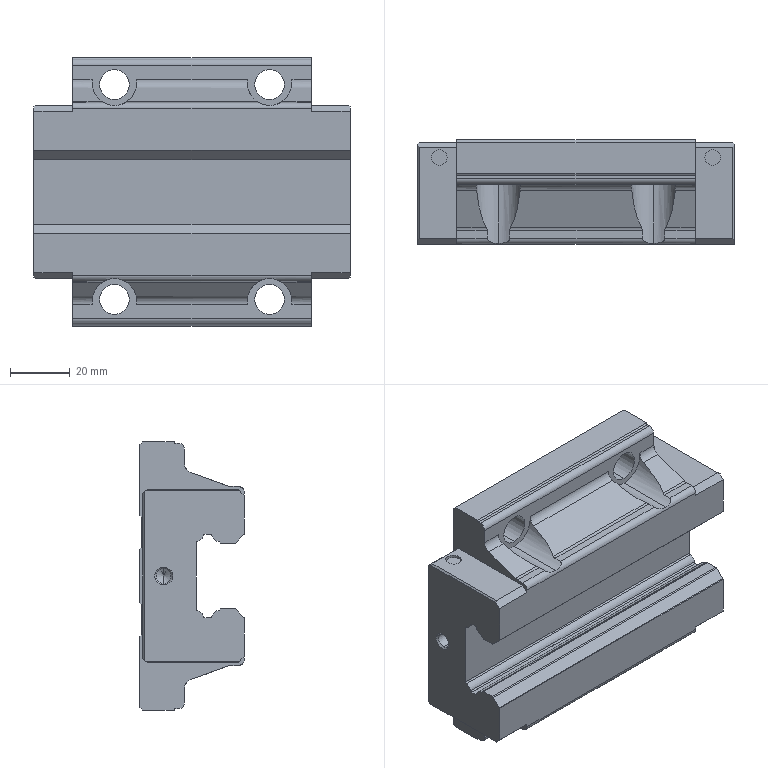Part | STEP file | J452-EBZ05-14-04-Part-1 | 1 solid | 149 faces | box 106 x 35 x 90 mm | volume 212002 mm3 | plane 76 | cylinder 65 | cone 8 | commonest cylinder face diameters 6 x12 5.2 x8 10 x8 15 x6 4 x4 4.917 x4